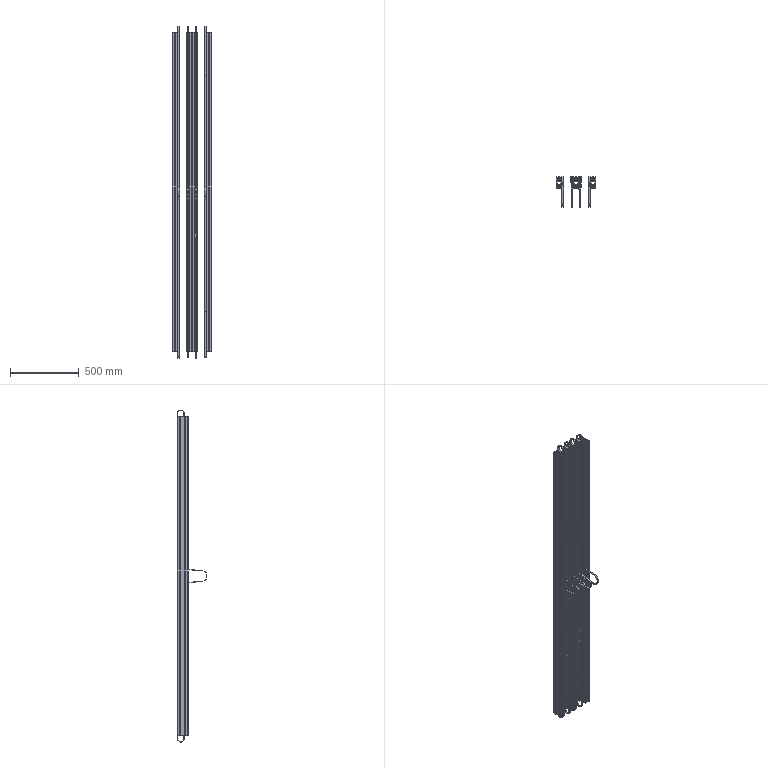Part | NX | features BREP 10 | 89 solids | 2695 faces | box 290 x 217.9 x 2421 mm | volume 12822795 mm3 | plane 1043 | cylinder 912 | cone 556 | torus 184 | commonest cylinder face diameters 8 x146 2 x140 3.3 x96 0.76 x60 11 x58 4.2 x52